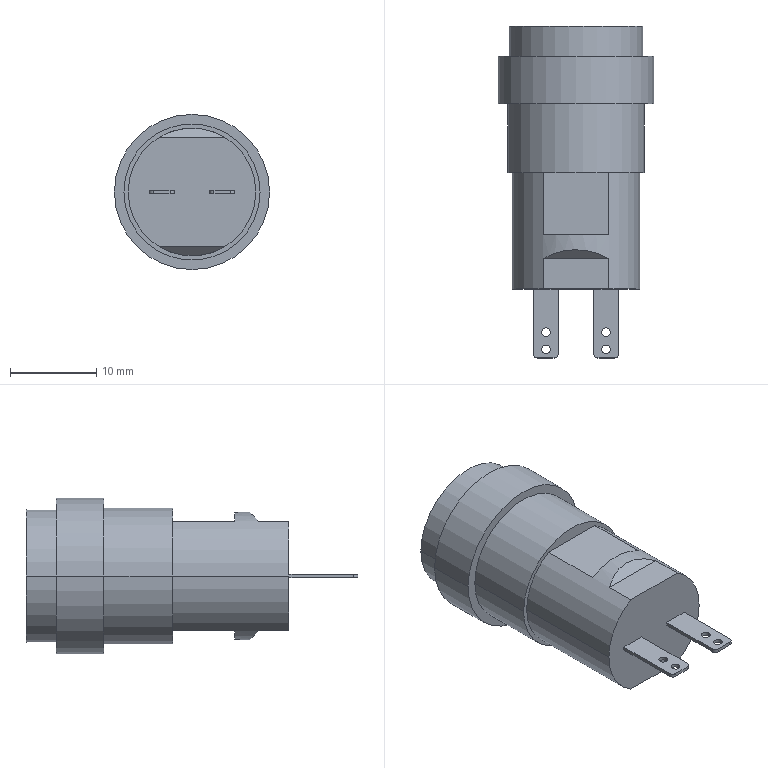Part | NX | 1 solid | 133 faces | box 18 x 38.5 x 18 mm | volume 5818 mm3 | plane 77 | cylinder 56 | commonest cylinder face diameters 1 x12 3 x6 5 x6 7 x6 9 x6 11 x6